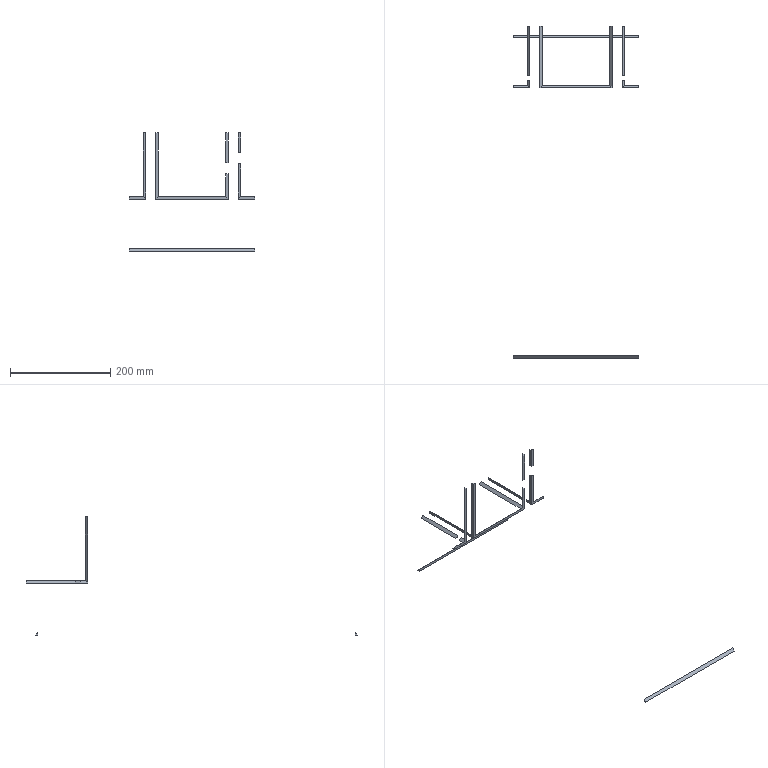Part | STEP file | MAT BAN CO LOGO 1_Welds | 9 solids | 61 faces | box 250 x 661.6 x 236 mm | volume 20450 mm3 | plane 61